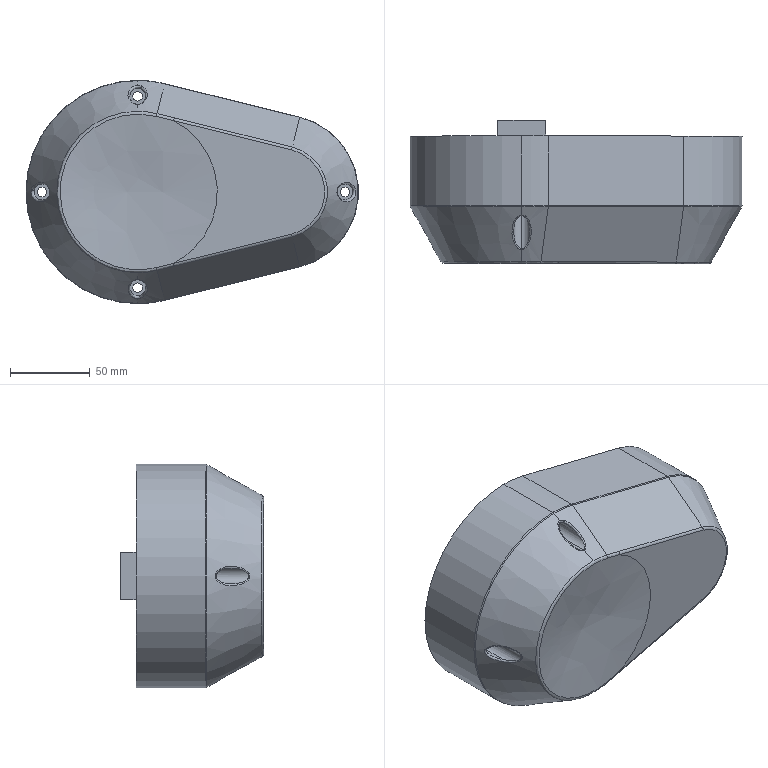Part | SolidWorks | features ICE 5, Fillet 2, Chamfer 1, CirPattern 1, Dome 1, Extrusion 1, PLine 1 | 1 solid | 60 faces | box 208.413 x 90 x 140 mm | volume 1586801 mm3 | cylinder 24 | plane 15 | spline 12 | torus 5 | cone 4 | commonest cylinder face diameters 6 x8 10 x8 4 x4 140 x3 96.825 x1